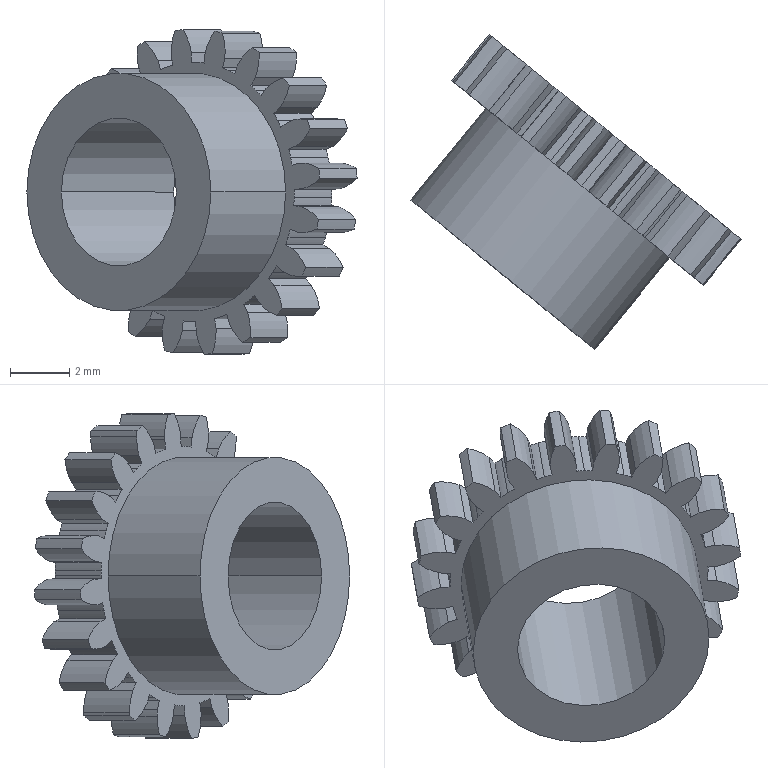Part | SolidWorks | features BaseBody 1 | 1 solid | 152 faces | box 11.141 x 10.637 x 10.961 mm | volume 236.653 mm3 | cylinder 109 | plane 43 | commonest cylinder face diameters 3.429 x44 4.52 x41 11 x20 5 x2 8 x2